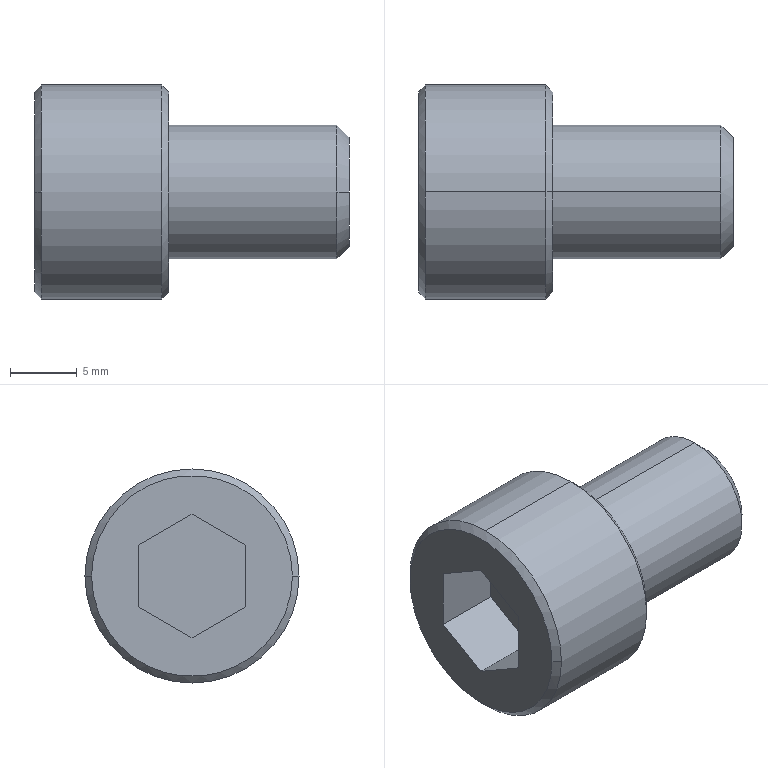Part | STEP file | TR_32x10-5 | 1 solid | 20 faces | box 23.5 x 16 x 16 mm | volume 2769 mm3 | plane 10 | cone 6 | cylinder 4 | commonest cylinder face diameters 10 x2 16 x2
STEP:
#1=CARTESIAN_POINT('',(0.,0.,0.));
#2=DIRECTION('',(0.,0.,1.));
#3=DIRECTION('',(1.,0.,0.));
#4=AXIS2_PLACEMENT_3D('',#1,#2,#3);
#5=CARTESIAN_POINT('',(-29.5,-14.,19.));
#6=VERTEX_POINT('',#5);
#7=CARTESIAN_POINT('',(-29.5,-22.,27.));
#8=VERTEX_POINT('',#7);
#9=CARTESIAN_POINT('',(-29.5,-22.,19.));
#10=DIRECTION('',(1.,0.,0.));
#11=DIRECTION('',(0.,0.,-1.));
#12=AXIS2_PLACEMENT_3D('',#9,#10,#11);
#13=CIRCLE('',#12,8.);
#14=CARTESIAN_POINT('',(-25.,-22.,19.));
#15=DIRECTION('',(1.,0.,0.));
#16=DIRECTION('',(0.,0.,-1.));
#17=AXIS2_PLACEMENT_3D('',#14,#15,#16);
#18=CYLINDRICAL_SURFACE('',#17,8.);
#19=CARTESIAN_POINT('',(0.,-4.5));
#20=DIRECTION('',(1.,0.));
#21=VECTOR('',#20,1.);
#22=LINE('',#19,#21);
#23=(GEOMETRIC_REPRESENTATION_CONTEXT(2)PARAMETRIC_REPRESENTATION_CONTEXT()REPRESENTATION_CONTEXT('',''));
#24=DEFINITIONAL_REPRESENTATION('',(#22),#23);
#25=PCURVE('',#18,#24);
#26=CARTESIAN_POINT('',(-29.5,-22.,19.));
#27=DIRECTION('',(1.,0.,0.));
#28=DIRECTION('',(0.,1.,0.));
#29=AXIS2_PLACEMENT_3D('',#26,#27,#28);
#30=CONICAL_SURFACE('',#29,8.,0.7854);
#31=CARTESIAN_POINT('',(-1.571,0.));
#32=DIRECTION('',(1.,0.));
#33=VECTOR('',#32,1.);
#34=LINE('',#31,#33);
#35=(GEOMETRIC_REPRESENTATION_CONTEXT(2)PARAMETRIC_REPRESENTATION_CONTEXT()REPRESENTATION_CONTEXT('',''));
#36=DEFINITIONAL_REPRESENTATION('',(#34),#35);
#37=PCURVE('',#30,#36);
#38=SURFACE_CURVE('',#13,(#25,#37),.PCURVE_S1.);
#39=EDGE_CURVE('',#6,#8,#38,.T.);
#40=ORIENTED_EDGE('',*,*,#39,.T.);
#41=CARTESIAN_POINT('',(-20.5,-22.,27.));
#42=VERTEX_POINT('',#41);
#43=CARTESIAN_POINT('',(-25.,-22.,27.));
#44=DIRECTION('',(1.,0.,0.));
#45=VECTOR('',#44,1.);
#46=LINE('',#43,#45);
#47=CARTESIAN_POINT('',(3.142,0.));
#48=DIRECTION('',(0.,1.));
#49=VECTOR('',#48,1.);
#50=LINE('',#47,#49);
#51=(GEOMETRIC_REPRESENTATION_CONTEXT(2)PARAMETRIC_REPRESENTATION_CONTEXT()REPRESENTATION_CONTEXT('',''));
#52=DEFINITIONAL_REPRESENTATION('',(#50),#51);
#53=PCURVE('',#18,#52);
#54=CARTESIAN_POINT('',(-25.,-22.,19.));
#55=DIRECTION('',(1.,0.,0.));
#56=DIRECTION('',(0.,0.,-1.));
#57=AXIS2_PLACEMENT_3D('',#54,#55,#56);
#58=CYLINDRICAL_SURFACE('',#57,8.);
#59=CARTESIAN_POINT('',(3.142,0.));
#60=DIRECTION('',(0.,1.));
#61=VECTOR('',#60,1.);
#62=LINE('',#59,#61);
#63=(GEOMETRIC_REPRESENTATION_CONTEXT(2)PARAMETRIC_REPRESENTATION_CONTEXT()REPRESENTATION_CONTEXT('',''));
#64=DEFINITIONAL_REPRESENTATION('',(#62),#63);
#65=PCURVE('',#58,#64);
#66=SURFACE_CURVE('',#46,(#53,#65),.PCURVE_S1.);
#67=EDGE_CURVE('',#8,#42,#66,.T.);
#68=ORIENTED_EDGE('',*,*,#67,.T.);
#69=CARTESIAN_POINT('',(-20.5,-22.,11.));
#70=VERTEX_POINT('',#69);
#71=CARTESIAN_POINT('',(-20.5,-22.,19.));
#72=DIRECTION('',(-1.,0.,0.));
#73=DIRECTION('',(0.,0.,-1.));
#74=AXIS2_PLACEMENT_3D('',#71,#72,#73);
#75=CIRCLE('',#74,8.);
#76=CARTESIAN_POINT('',(6.283,4.5));
#77=DIRECTION('',(-1.,0.));
#78=VECTOR('',#77,1.);
#79=LINE('',#76,#78);
#80=(GEOMETRIC_REPRESENTATION_CONTEXT(2)PARAMETRIC_REPRESENTATION_CONTEXT()REPRESENTATION_CONTEXT('',''));
#81=DEFINITIONAL_REPRESENTATION('',(#79),#80);
#82=PCURVE('',#18,#81);
#83=CARTESIAN_POINT('',(-20.5,-22.,19.));
#84=DIRECTION('',(-1.,0.,0.));
#85=DIRECTION('',(0.,0.,1.));
#86=AXIS2_PLACEMENT_3D('',#83,#84,#85);
#87=CONICAL_SURFACE('',#86,8.,0.7854);
#88=CARTESIAN_POINT('',(-3.142,0.));
#89=DIRECTION('',(1.,0.));
#90=VECTOR('',#89,1.);
#91=LINE('',#88,#90);
#92=(GEOMETRIC_REPRESENTATION_CONTEXT(2)PARAMETRIC_REPRESENTATION_CONTEXT()REPRESENTATION_CONTEXT('',''));
#93=DEFINITIONAL_REPRESENTATION('',(#91),#92);
#94=PCURVE('',#87,#93);
#95=SURFACE_CURVE('',#75,(#82,#94),.PCURVE_S1.);
#96=EDGE_CURVE('',#42,#70,#95,.T.);
#97=ORIENTED_EDGE('',*,*,#96,.T.);
#98=CARTESIAN_POINT('',(-29.5,-22.,11.));
#99=VERTEX_POINT('',#98);
#100=CARTESIAN_POINT('',(-25.,-22.,11.));
#101=DIRECTION('',(1.,0.,0.));
#102=VECTOR('',#101,1.);
#103=LINE('',#100,#102);
#104=CARTESIAN_POINT('',(0.,0.));
#105=DIRECTION('',(0.,1.));
#106=VECTOR('',#105,1.);
#107=LINE('',#104,#106);
#108=(GEOMETRIC_REPRESENTATION_CONTEXT(2)PARAMETRIC_REPRESENTATION_CONTEXT()REPRESENTATION_CONTEXT('',''));
#109=DEFINITIONAL_REPRESENTATION('',(#107),#108);
#110=PCURVE('',#18,#109);
#111=CARTESIAN_POINT('',(6.283,0.));
#112=DIRECTION('',(0.,1.));
#113=VECTOR('',#112,1.);
#114=LINE('',#111,#113);
#115=(GEOMETRIC_REPRESENTATION_CONTEXT(2)PARAMETRIC_REPRESENTATION_CONTEXT()REPRESENTATION_CONTEXT('',''));
#116=DEFINITIONAL_REPRESENTATION('',(#114),#115);
#117=PCURVE('',#58,#116);
#118=SURFACE_CURVE('',#103,(#110,#117),.PCURVE_S1.);
#119=EDGE_CURVE('',#99,#70,#118,.T.);
#120=ORIENTED_EDGE('',*,*,#119,.F.);
#121=CARTESIAN_POINT('',(-29.5,-22.,19.));
#122=DIRECTION('',(1.,0.,0.));
#123=DIRECTION('',(0.,0.,-1.));
#124=AXIS2_PLACEMENT_3D('',#121,#122,#123);
#125=CIRCLE('',#124,8.);
#126=CARTESIAN_POINT('',(0.,-4.5));
#127=DIRECTION('',(1.,0.));
#128=VECTOR('',#127,1.);
#129=LINE('',#126,#128);
#130=(GEOMETRIC_REPRESENTATION_CONTEXT(2)PARAMETRIC_REPRESENTATION_CONTEXT()REPRESENTATION_CONTEXT('',''));
#131=DEFINITIONAL_REPRESENTATION('',(#129),#130);
#132=PCURVE('',#18,#131);
#133=CARTESIAN_POINT('',(-29.5,-22.,19.));
#134=DIRECTION('',(1.,0.,0.));
#135=DIRECTION('',(0.,1.,0.));
#136=AXIS2_PLACEMENT_3D('',#133,#134,#135);
#137=CONICAL_SURFACE('',#136,8.,0.7854);
#138=CARTESIAN_POINT('',(4.712,0.));
#139=DIRECTION('',(1.,0.));
#140=VECTOR('',#139,1.);
#141=LINE('',#138,#140);
#142=(GEOMETRIC_REPRESENTATION_CONTEXT(2)PARAMETRIC_REPRESENTATION_CONTEXT()REPRESENTATION_CONTEXT('',''));
#143=DEFINITIONAL_REPRESENTATION('',(#141),#142);
#144=PCURVE('',#137,#143);
#145=SURFACE_CURVE('',#125,(#132,#144),.PCURVE_S1.);
#146=EDGE_CURVE('',#99,#6,#145,.T.);
#147=ORIENTED_EDGE('',*,*,#146,.T.);
#148=EDGE_LOOP('',(#40,#68,#97,#120,#147));
#149=FACE_BOUND('',#148,.T.);
#150=ADVANCED_FACE('',(#149),#18,.T.);
#151=CARTESIAN_POINT('',(-30.,-14.5,19.));
#152=VERTEX_POINT('',#151);
#153=CARTESIAN_POINT('',(-30.,-29.5,19.));
#154=VERTEX_POINT('',#153);
#155=CARTESIAN_POINT('',(-30.,-22.,19.));
#156=DIRECTION('',(1.,0.,0.));
#157=DIRECTION('',(0.,1.,0.));
#158=AXIS2_PLACEMENT_3D('',#155,#156,#157);
#159=CIRCLE('',#158,7.5);
#160=CARTESIAN_POINT('',(0.,-0.5));
#161=DIRECTION('',(1.,0.));
#162=VECTOR('',#161,1.);
#163=LINE('',#160,#162);
#164=(GEOMETRIC_REPRESENTATION_CONTEXT(2)PARAMETRIC_REPRESENTATION_CONTEXT()REPRESENTATION_CONTEXT('',''));
#165=DEFINITIONAL_REPRESENTATION('',(#163),#164);
#166=PCURVE('',#30,#165);
#167=CARTESIAN_POINT('',(-30.,-22.,22.75));
#168=DIRECTION('',(-1.,0.,0.));
#169=DIRECTION('',(0.,0.,1.));
#170=AXIS2_PLACEMENT_3D('',#167,#168,#169);
#171=PLANE('',#170);
#172=CARTESIAN_POINT('',(-3.75,7.5));
#173=CARTESIAN_POINT('',(9.24,7.5));
#174=CARTESIAN_POINT('',(2.745,-3.75));
#175=CARTESIAN_POINT('',(-3.75,-15.));
#176=CARTESIAN_POINT('',(-10.245,-3.75));
#177=CARTESIAN_POINT('',(-16.74,7.5));
#178=CARTESIAN_POINT('',(-3.75,7.5));
#179=(BOUNDED_CURVE()B_SPLINE_CURVE(2,(#172,#173,#174,#175,#176,#177,#178),.UNSPECIFIED.,.T.,.F.)B_SPLINE_CURVE_WITH_KNOTS((1,2,2,2,2,1),(-2.094,0.,2.094,4.189,6.283,8.378),.UNSPECIFIED.)CURVE()GEOMETRIC_REPRESENTATION_ITEM()RATIONAL_B_SPLINE_CURVE((1.,0.5,1.,0.5,1.,0.5,1.))REPRESENTATION_ITEM(''));
#180=(GEOMETRIC_REPRESENTATION_CONTEXT(2)PARAMETRIC_REPRESENTATION_CONTEXT()REPRESENTATION_CONTEXT('',''));
#181=DEFINITIONAL_REPRESENTATION('',(#179),#180);
#182=PCURVE('',#171,#181);
#183=SURFACE_CURVE('',#159,(#166,#182),.PCURVE_S1.);
#184=EDGE_CURVE('',#152,#154,#183,.T.);
#185=ORIENTED_EDGE('',*,*,#184,.T.);
#186=CARTESIAN_POINT('',(-29.5,-30.,19.));
#187=VERTEX_POINT('',#186);
#188=CARTESIAN_POINT('',(-29.5,-30.,19.));
#189=DIRECTION('',(0.7071,-0.7071,0.));
#190=VECTOR('',#189,1.);
#191=LINE('',#188,#190);
#192=CARTESIAN_POINT('',(3.142,0.));
#193=DIRECTION('',(0.,1.));
#194=VECTOR('',#193,1.);
#195=LINE('',#192,#194);
#196=(GEOMETRIC_REPRESENTATION_CONTEXT(2)PARAMETRIC_REPRESENTATION_CONTEXT()REPRESENTATION_CONTEXT('',''));
#197=DEFINITIONAL_REPRESENTATION('',(#195),#196);
#198=PCURVE('',#30,#197);
#199=CARTESIAN_POINT('',(3.142,0.));
#200=DIRECTION('',(0.,1.));
#201=VECTOR('',#200,1.);
#202=LINE('',#199,#201);
#203=(GEOMETRIC_REPRESENTATION_CONTEXT(2)PARAMETRIC_REPRESENTATION_CONTEXT()REPRESENTATION_CONTEXT('',''));
#204=DEFINITIONAL_REPRESENTATION('',(#202),#203);
#205=PCURVE('',#137,#204);
#206=SURFACE_CURVE('',#191,(#198,#205),.PCURVE_S1.);
#207=EDGE_CURVE('',#154,#187,#206,.T.);
#208=ORIENTED_EDGE('',*,*,#207,.T.);
#209=CARTESIAN_POINT('',(-29.5,-22.,19.));
#210=DIRECTION('',(1.,0.,0.));
#211=DIRECTION('',(0.,0.,-1.));
#212=AXIS2_PLACEMENT_3D('',#209,#210,#211);
#213=CIRCLE('',#212,8.);
#214=CARTESIAN_POINT('',(-1.571,0.));
#215=DIRECTION('',(1.,0.));
#216=VECTOR('',#215,1.);
#217=LINE('',#214,#216);
#218=(GEOMETRIC_REPRESENTATION_CONTEXT(2)PARAMETRIC_REPRESENTATION_CONTEXT()REPRESENTATION_CONTEXT('',''));
#219=DEFINITIONAL_REPRESENTATION('',(#217),#218);
#220=PCURVE('',#30,#219);
#221=CARTESIAN_POINT('',(0.,-4.5));
#222=DIRECTION('',(1.,0.));
#223=VECTOR('',#222,1.);
#224=LINE('',#221,#223);
#225=(GEOMETRIC_REPRESENTATION_CONTEXT(2)PARAMETRIC_REPRESENTATION_CONTEXT()REPRESENTATION_CONTEXT('',''));
#226=DEFINITIONAL_REPRESENTATION('',(#224),#225);
#227=PCURVE('',#58,#226);
#228=SURFACE_CURVE('',#213,(#220,#227),.PCURVE_S1.);
#229=EDGE_CURVE('',#8,#187,#228,.T.);
#230=ORIENTED_EDGE('',*,*,#229,.F.);
#231=ORIENTED_EDGE('',*,*,#39,.F.);
#232=CARTESIAN_POINT('',(-29.5,-14.,19.));
#233=DIRECTION('',(0.7071,0.7071,0.));
#234=VECTOR('',#233,1.);
#235=LINE('',#232,#234);
#236=CARTESIAN_POINT('',(0.,0.));
#237=DIRECTION('',(0.,1.));
#238=VECTOR('',#237,1.);
#239=LINE('',#236,#238);
#240=(GEOMETRIC_REPRESENTATION_CONTEXT(2)PARAMETRIC_REPRESENTATION_CONTEXT()REPRESENTATION_CONTEXT('',''));
#241=DEFINITIONAL_REPRESENTATION('',(#239),#240);
#242=PCURVE('',#30,#241);
#243=CARTESIAN_POINT('',(6.283,0.));
#244=DIRECTION('',(0.,1.));
#245=VECTOR('',#244,1.);
#246=LINE('',#243,#245);
#247=(GEOMETRIC_REPRESENTATION_CONTEXT(2)PARAMETRIC_REPRESENTATION_CONTEXT()REPRESENTATION_CONTEXT('',''));
#248=DEFINITIONAL_REPRESENTATION('',(#246),#247);
#249=PCURVE('',#137,#248);
#250=SURFACE_CURVE('',#235,(#242,#249),.PCURVE_S1.);
#251=EDGE_CURVE('',#152,#6,#250,.T.);
#252=ORIENTED_EDGE('',*,*,#251,.F.);
#253=EDGE_LOOP('',(#185,#208,#230,#231,#252));
#254=FACE_BOUND('',#253,.T.);
#255=ADVANCED_FACE('',(#254),#30,.T.);
#256=CARTESIAN_POINT('',(-20.,-22.,26.5));
#257=VERTEX_POINT('',#256);
#258=CARTESIAN_POINT('',(-20.,-22.,11.5));
#259=VERTEX_POINT('',#258);
#260=CARTESIAN_POINT('',(-20.,-22.,19.));
#261=DIRECTION('',(-1.,0.,0.));
#262=DIRECTION('',(0.,0.,1.));
#263=AXIS2_PLACEMENT_3D('',#260,#261,#262);
#264=CIRCLE('',#263,7.5);
#265=CARTESIAN_POINT('',(0.,-0.5));
#266=DIRECTION('',(1.,0.));
#267=VECTOR('',#266,1.);
#268=LINE('',#265,#267);
#269=(GEOMETRIC_REPRESENTATION_CONTEXT(2)PARAMETRIC_REPRESENTATION_CONTEXT()REPRESENTATION_CONTEXT('',''));
#270=DEFINITIONAL_REPRESENTATION('',(#268),#269);
#271=PCURVE('',#87,#270);
#272=CARTESIAN_POINT('',(-20.,-22.,25.25));
#273=DIRECTION('',(1.,0.,0.));
#274=DIRECTION('',(0.,0.,-1.));
#275=AXIS2_PLACEMENT_3D('',#272,#273,#274);
#276=PLANE('',#275);
#277=CARTESIAN_POINT('',(-1.25,0.));
#278=CARTESIAN_POINT('',(-1.25,12.99));
#279=CARTESIAN_POINT('',(10.,6.495));
#280=CARTESIAN_POINT('',(21.25,0.));
#281=CARTESIAN_POINT('',(10.,-6.495));
#282=CARTESIAN_POINT('',(-1.25,-12.99));
#283=CARTESIAN_POINT('',(-1.25,0.));
#284=(BOUNDED_CURVE()B_SPLINE_CURVE(2,(#277,#278,#279,#280,#281,#282,#283),.UNSPECIFIED.,.T.,.F.)B_SPLINE_CURVE_WITH_KNOTS((1,2,2,2,2,1),(-2.094,0.,2.094,4.189,6.283,8.378),.UNSPECIFIED.)CURVE()GEOMETRIC_REPRESENTATION_ITEM()RATIONAL_B_SPLINE_CURVE((1.,0.5,1.,0.5,1.,0.5,1.))REPRESENTATION_ITEM(''));
#285=(GEOMETRIC_REPRESENTATION_CONTEXT(2)PARAMETRIC_REPRESENTATION_CONTEXT()REPRESENTATION_CONTEXT('',''));
#286=DEFINITIONAL_REPRESENTATION('',(#284),#285);
#287=PCURVE('',#276,#286);
#288=SURFACE_CURVE('',#264,(#271,#287),.PCURVE_S1.);
#289=EDGE_CURVE('',#257,#259,#288,.T.);
#290=ORIENTED_EDGE('',*,*,#289,.T.);
#291=CARTESIAN_POINT('',(-20.5,-22.,11.));
#292=DIRECTION('',(-0.7071,0.,-0.7071));
#293=VECTOR('',#292,1.);
#294=LINE('',#291,#293);
#295=CARTESIAN_POINT('',(3.142,0.));
#296=DIRECTION('',(0.,1.));
#297=VECTOR('',#296,1.);
#298=LINE('',#295,#297);
#299=(GEOMETRIC_REPRESENTATION_CONTEXT(2)PARAMETRIC_REPRESENTATION_CONTEXT()REPRESENTATION_CONTEXT('',''));
#300=DEFINITIONAL_REPRESENTATION('',(#298),#299);
#301=PCURVE('',#87,#300);
#302=CARTESIAN_POINT('',(-20.5,-22.,19.));
#303=DIRECTION('',(-1.,0.,0.));
#304=DIRECTION('',(0.,0.,1.));
#305=AXIS2_PLACEMENT_3D('',#302,#303,#304);
#306=CONICAL_SURFACE('',#305,8.,0.7854);
#307=CARTESIAN_POINT('',(3.142,0.));
#308=DIRECTION('',(0.,1.));
#309=VECTOR('',#308,1.);
#310=LINE('',#307,#309);
#311=(GEOMETRIC_REPRESENTATION_CONTEXT(2)PARAMETRIC_REPRESENTATION_CONTEXT()REPRESENTATION_CONTEXT('',''));
#312=DEFINITIONAL_REPRESENTATION('',(#310),#311);
#313=PCURVE('',#306,#312);
#314=SURFACE_CURVE('',#294,(#301,#313),.PCURVE_S1.);
#315=EDGE_CURVE('',#259,#70,#314,.T.);
#316=ORIENTED_EDGE('',*,*,#315,.T.);
#317=ORIENTED_EDGE('',*,*,#96,.F.);
#318=CARTESIAN_POINT('',(-20.5,-22.,27.));
#319=DIRECTION('',(-0.7071,0.,0.7071));
#320=VECTOR('',#319,1.);
#321=LINE('',#318,#320);
#322=CARTESIAN_POINT('',(0.,0.));
#323=DIRECTION('',(0.,1.));
#324=VECTOR('',#323,1.);
#325=LINE('',#322,#324);
#326=(GEOMETRIC_REPRESENTATION_CONTEXT(2)PARAMETRIC_REPRESENTATION_CONTEXT()REPRESENTATION_CONTEXT('',''));
#327=DEFINITIONAL_REPRESENTATION('',(#325),#326);
#328=PCURVE('',#87,#327);
#329=CARTESIAN_POINT('',(6.283,0.));
#330=DIRECTION('',(0.,1.));
#331=VECTOR('',#330,1.);
#332=LINE('',#329,#331);
#333=(GEOMETRIC_REPRESENTATION_CONTEXT(2)PARAMETRIC_REPRESENTATION_CONTEXT()REPRESENTATION_CONTEXT('',''));
#334=DEFINITIONAL_REPRESENTATION('',(#332),#333);
#335=PCURVE('',#306,#334);
#336=SURFACE_CURVE('',#321,(#328,#335),.PCURVE_S1.);
#337=EDGE_CURVE('',#257,#42,#336,.T.);
#338=ORIENTED_EDGE('',*,*,#337,.F.);
#339=EDGE_LOOP('',(#290,#316,#317,#338));
#340=FACE_BOUND('',#339,.T.);
#341=ADVANCED_FACE('',(#340),#87,.T.);
#342=CARTESIAN_POINT('',(-20.,-22.,24.));
#343=VERTEX_POINT('',#342);
#344=CARTESIAN_POINT('',(-20.,-22.,14.));
#345=VERTEX_POINT('',#344);
#346=CARTESIAN_POINT('',(-20.,-22.,19.));
#347=DIRECTION('',(-1.,0.,0.));
#348=DIRECTION('',(0.,0.,-1.));
#349=AXIS2_PLACEMENT_3D('',#346,#347,#348);
#350=CIRCLE('',#349,5.);
#351=CARTESIAN_POINT('',(-13.71,-22.,19.));
#352=DIRECTION('',(1.,0.,0.));
#353=DIRECTION('',(0.,0.,-1.));
#354=AXIS2_PLACEMENT_3D('',#351,#352,#353);
#355=CYLINDRICAL_SURFACE('',#354,5.);
#356=CARTESIAN_POINT('',(6.283,-6.29));
#357=DIRECTION('',(-1.,0.));
#358=VECTOR('',#357,1.);
#359=LINE('',#356,#358);
#360=(GEOMETRIC_REPRESENTATION_CONTEXT(2)PARAMETRIC_REPRESENTATION_CONTEXT()REPRESENTATION_CONTEXT('',''));
#361=DEFINITIONAL_REPRESENTATION('',(#359),#360);
#362=PCURVE('',#355,#361);
#363=CARTESIAN_POINT('',(11.25,0.));
#364=CARTESIAN_POINT('',(11.25,-8.66));
#365=CARTESIAN_POINT('',(3.75,-4.33));
#366=CARTESIAN_POINT('',(-3.75,0.));
#367=CARTESIAN_POINT('',(3.75,4.33));
#368=CARTESIAN_POINT('',(11.25,8.66));
#369=CARTESIAN_POINT('',(11.25,0.));
#370=(BOUNDED_CURVE()B_SPLINE_CURVE(2,(#363,#364,#365,#366,#367,#368,#369),.UNSPECIFIED.,.T.,.F.)B_SPLINE_CURVE_WITH_KNOTS((1,2,2,2,2,1),(-2.094,0.,2.094,4.189,6.283,8.378),.UNSPECIFIED.)CURVE()GEOMETRIC_REPRESENTATION_ITEM()RATIONAL_B_SPLINE_CURVE((1.,0.5,1.,0.5,1.,0.5,1.))REPRESENTATION_ITEM(''));
#371=(GEOMETRIC_REPRESENTATION_CONTEXT(2)PARAMETRIC_REPRESENTATION_CONTEXT()REPRESENTATION_CONTEXT('',''));
#372=DEFINITIONAL_REPRESENTATION('',(#370),#371);
#373=PCURVE('',#276,#372);
#374=SURFACE_CURVE('',#350,(#362,#373),.PCURVE_S1.);
#375=EDGE_CURVE('',#343,#345,#374,.T.);
#376=ORIENTED_EDGE('',*,*,#375,.F.);
#377=CARTESIAN_POINT('',(-7.42,-22.,24.));
#378=VERTEX_POINT('',#377);
#379=CARTESIAN_POINT('',(-13.71,-22.,24.));
#380=DIRECTION('',(1.,0.,0.));
#381=VECTOR('',#380,1.);
#382=LINE('',#379,#381);
#383=CARTESIAN_POINT('',(3.142,0.));
#384=DIRECTION('',(0.,1.));
#385=VECTOR('',#384,1.);
#386=LINE('',#383,#385);
#387=(GEOMETRIC_REPRESENTATION_CONTEXT(2)PARAMETRIC_REPRESENTATION_CONTEXT()REPRESENTATION_CONTEXT('',''));
#388=DEFINITIONAL_REPRESENTATION('',(#386),#387);
#389=PCURVE('',#355,#388);
#390=CARTESIAN_POINT('',(-13.71,-22.,19.));
#391=DIRECTION('',(1.,0.,0.));
#392=DIRECTION('',(0.,0.,-1.));
#393=AXIS2_PLACEMENT_3D('',#390,#391,#392);
#394=CYLINDRICAL_SURFACE('',#393,5.);
#395=CARTESIAN_POINT('',(3.142,0.));
#396=DIRECTION('',(0.,1.));
#397=VECTOR('',#396,1.);
#398=LINE('',#395,#397);
#399=(GEOMETRIC_REPRESENTATION_CONTEXT(2)PARAMETRIC_REPRESENTATION_CONTEXT()REPRESENTATION_CONTEXT('',''));
#400=DEFINITIONAL_REPRESENTATION('',(#398),#399);
#401=PCURVE('',#394,#400);
#402=SURFACE_CURVE('',#382,(#389,#401),.PCURVE_S1.);
#403=EDGE_CURVE('',#343,#378,#402,.T.);
#404=ORIENTED_EDGE('',*,*,#403,.T.);
#405=CARTESIAN_POINT('',(-7.42,-17.,19.));
#406=VERTEX_POINT('',#405);
#407=CARTESIAN_POINT('',(-7.42,-22.,19.));
#408=DIRECTION('',(-1.,0.,0.));
#409=DIRECTION('',(0.,0.,-1.));
#410=AXIS2_PLACEMENT_3D('',#407,#408,#409);
#411=CIRCLE('',#410,5.);
#412=CARTESIAN_POINT('',(6.283,6.29));
#413=DIRECTION('',(-1.,0.));
#414=VECTOR('',#413,1.);
#415=LINE('',#412,#414);
#416=(GEOMETRIC_REPRESENTATION_CONTEXT(2)PARAMETRIC_REPRESENTATION_CONTEXT()REPRESENTATION_CONTEXT('',''));
#417=DEFINITIONAL_REPRESENTATION('',(#415),#416);
#418=PCURVE('',#355,#417);
#419=CARTESIAN_POINT('',(-7.42,-22.,19.));
#420=DIRECTION('',(-1.,0.,0.));
#421=DIRECTION('',(0.,-1.,0.));
#422=AXIS2_PLACEMENT_3D('',#419,#420,#421);
#423=CONICAL_SURFACE('',#422,5.,0.7854);
#424=CARTESIAN_POINT('',(-1.571,0.));
#425=DIRECTION('',(1.,0.));
#426=VECTOR('',#425,1.);
#427=LINE('',#424,#426);
#428=(GEOMETRIC_REPRESENTATION_CONTEXT(2)PARAMETRIC_REPRESENTATION_CONTEXT()REPRESENTATION_CONTEXT('',''));
#429=DEFINITIONAL_REPRESENTATION('',(#427),#428);
#430=PCURVE('',#423,#429);
#431=SURFACE_CURVE('',#411,(#418,#430),.PCURVE_S1.);
#432=EDGE_CURVE('',#378,#406,#431,.T.);
#433=ORIENTED_EDGE('',*,*,#432,.T.);
#434=CARTESIAN_POINT('',(-7.42,-22.,14.));
#435=VERTEX_POINT('',#434);
#436=CARTESIAN_POINT('',(-7.42,-22.,19.));
#437=DIRECTION('',(-1.,0.,0.));
#438=DIRECTION('',(0.,0.,-1.));
#439=AXIS2_PLACEMENT_3D('',#436,#437,#438);
#440=CIRCLE('',#439,5.);
#441=CARTESIAN_POINT('',(6.283,6.29));
#442=DIRECTION('',(-1.,0.));
#443=VECTOR('',#442,1.);
#444=LINE('',#441,#443);
#445=(GEOMETRIC_REPRESENTATION_CONTEXT(2)PARAMETRIC_REPRESENTATION_CONTEXT()REPRESENTATION_CONTEXT('',''));
#446=DEFINITIONAL_REPRESENTATION('',(#444),#445);
#447=PCURVE('',#355,#446);
#448=CARTESIAN_POINT('',(-7.42,-22.,19.));
#449=DIRECTION('',(-1.,0.,0.));
#450=DIRECTION('',(0.,-1.,0.));
#451=AXIS2_PLACEMENT_3D('',#448,#449,#450);
#452=CONICAL_SURFACE('',#451,5.,0.7854);
#453=CARTESIAN_POINT('',(-1.571,0.));
#454=DIRECTION('',(1.,0.));
#455=VECTOR('',#454,1.);
#456=LINE('',#453,#455);
#457=(GEOMETRIC_REPRESENTATION_CONTEXT(2)PARAMETRIC_REPRESENTATION_CONTEXT()REPRESENTATION_CONTEXT('',''));
#458=DEFINITIONAL_REPRESENTATION('',(#456),#457);
#459=PCURVE('',#452,#458);
#460=SURFACE_CURVE('',#440,(#447,#459),.PCURVE_S1.);
#461=EDGE_CURVE('',#406,#435,#460,.T.);
#462=ORIENTED_EDGE('',*,*,#461,.T.);
#463=CARTESIAN_POINT('',(-13.71,-22.,14.));
#464=DIRECTION('',(1.,0.,0.));
#465=VECTOR('',#464,1.);
#466=LINE('',#463,#465);
#467=CARTESIAN_POINT('',(0.,0.));
#468=DIRECTION('',(0.,1.));
#469=VECTOR('',#468,1.);
#470=LINE('',#467,#469);
#471=(GEOMETRIC_REPRESENTATION_CONTEXT(2)PARAMETRIC_REPRESENTATION_CONTEXT()REPRESENTATION_CONTEXT('',''));
#472=DEFINITIONAL_REPRESENTATION('',(#470),#471);
#473=PCURVE('',#355,#472);
#474=CARTESIAN_POINT('',(6.283,0.));
#475=DIRECTION('',(0.,1.));
#476=VECTOR('',#475,1.);
#477=LINE('',#474,#476);
#478=(GEOMETRIC_REPRESENTATION_CONTEXT(2)PARAMETRIC_REPRESENTATION_CONTEXT()REPRESENTATION_CONTEXT('',''));
#479=DEFINITIONAL_REPRESENTATION('',(#477),#478);
#480=PCURVE('',#394,#479);
#481=SURFACE_CURVE('',#466,(#473,#480),.PCURVE_S1.);
#482=EDGE_CURVE('',#345,#435,#481,.T.);
#483=ORIENTED_EDGE('',*,*,#482,.F.);
#484=EDGE_LOOP('',(#376,#404,#433,#462,#483));
#485=FACE_BOUND('',#484,.T.);
#486=ADVANCED_FACE('',(#485),#355,.T.);
#487=CARTESIAN_POINT('',(-6.5,-26.08,19.));
#488=VERTEX_POINT('',#487);
#489=CARTESIAN_POINT('',(-6.5,-17.92,19.));
#490=VERTEX_POINT('',#489);
#491=CARTESIAN_POINT('',(-6.5,-22.,19.));
#492=DIRECTION('',(-1.,0.,0.));
#493=DIRECTION('',(0.,-1.,0.));
#494=AXIS2_PLACEMENT_3D('',#491,#492,#493);
#495=CIRCLE('',#494,4.08);
#496=CARTESIAN_POINT('',(0.,-0.92));
#497=DIRECTION('',(1.,0.));
#498=VECTOR('',#497,1.);
#499=LINE('',#496,#498);
#500=(GEOMETRIC_REPRESENTATION_CONTEXT(2)PARAMETRIC_REPRESENTATION_CONTEXT()REPRESENTATION_CONTEXT('',''));
#501=DEFINITIONAL_REPRESENTATION('',(#499),#500);
#502=PCURVE('',#423,#501);
#503=CARTESIAN_POINT('',(-6.5,-22.,21.04));
#504=DIRECTION('',(1.,0.,0.));
#505=DIRECTION('',(0.,0.,-1.));
#506=AXIS2_PLACEMENT_3D('',#503,#504,#505);
#507=PLANE('',#506);
#508=CARTESIAN_POINT('',(2.04,-4.08));
#509=CARTESIAN_POINT('',(-5.027,-4.08));
#510=CARTESIAN_POINT('',(-1.493,2.04));
#511=CARTESIAN_POINT('',(2.04,8.16));
#512=CARTESIAN_POINT('',(5.573,2.04));
#513=CARTESIAN_POINT('',(9.107,-4.08));
#514=CARTESIAN_POINT('',(2.04,-4.08));
#515=(BOUNDED_CURVE()B_SPLINE_CURVE(2,(#508,#509,#510,#511,#512,#513,#514),.UNSPECIFIED.,.T.,.F.)B_SPLINE_CURVE_WITH_KNOTS((1,2,2,2,2,1),(-2.094,0.,2.094,4.189,6.283,8.378),.UNSPECIFIED.)CURVE()GEOMETRIC_REPRESENTATION_ITEM()RATIONAL_B_SPLINE_CURVE((1.,0.5,1.,0.5,1.,0.5,1.))REPRESENTATION_ITEM(''));
#516=(GEOMETRIC_REPRESENTATION_CONTEXT(2)PARAMETRIC_REPRESENTATION_CONTEXT()REPRESENTATION_CONTEXT('',''));
#517=DEFINITIONAL_REPRESENTATION('',(#515),#516);
#518=PCURVE('',#507,#517);
#519=SURFACE_CURVE('',#495,(#502,#518),.PCURVE_S1.);
#520=EDGE_CURVE('',#488,#490,#519,.T.);
#521=ORIENTED_EDGE('',*,*,#520,.T.);
#522=CARTESIAN_POINT('',(-7.42,-17.,19.));
#523=DIRECTION('',(-0.7071,0.7071,0.));
#524=VECTOR('',#523,1.);
#525=LINE('',#522,#524);
#526=CARTESIAN_POINT('',(3.142,0.));
#527=DIRECTION('',(0.,1.));
#528=VECTOR('',#527,1.);
#529=LINE('',#526,#528);
#530=(GEOMETRIC_REPRESENTATION_CONTEXT(2)PARAMETRIC_REPRESENTATION_CONTEXT()REPRESENTATION_CONTEXT('',''));
#531=DEFINITIONAL_REPRESENTATION('',(#529),#530);
#532=PCURVE('',#423,#531);
#533=CARTESIAN_POINT('',(3.142,0.));
#534=DIRECTION('',(0.,1.));
#535=VECTOR('',#534,1.);
#536=LINE('',#533,#535);
#537=(GEOMETRIC_REPRESENTATION_CONTEXT(2)PARAMETRIC_REPRESENTATION_CONTEXT()REPRESENTATION_CONTEXT('',''));
#538=DEFINITIONAL_REPRESENTATION('',(#536),#537);
#539=PCURVE('',#452,#538);
#540=SURFACE_CURVE('',#525,(#532,#539),.PCURVE_S1.);
#541=EDGE_CURVE('',#490,#406,#540,.T.);
#542=ORIENTED_EDGE('',*,*,#541,.T.);
#543=ORIENTED_EDGE('',*,*,#432,.F.);
#544=CARTESIAN_POINT('',(-7.42,-27.,19.));
#545=VERTEX_POINT('',#544);
#546=CARTESIAN_POINT('',(-7.42,-22.,19.));
#547=DIRECTION('',(-1.,0.,0.));
#548=DIRECTION('',(0.,0.,-1.));
#549=AXIS2_PLACEMENT_3D('',#546,#547,#548);
#550=CIRCLE('',#549,5.);
#551=CARTESIAN_POINT('',(-1.571,0.));
#552=DIRECTION('',(1.,0.));
#553=VECTOR('',#552,1.);
#554=LINE('',#551,#553);
#555=(GEOMETRIC_REPRESENTATION_CONTEXT(2)PARAMETRIC_REPRESENTATION_CONTEXT()REPRESENTATION_CONTEXT('',''));
#556=DEFINITIONAL_REPRESENTATION('',(#554),#555);
#557=PCURVE('',#423,#556);
#558=CARTESIAN_POINT('',(6.283,6.29));
#559=DIRECTION('',(-1.,0.));
#560=VECTOR('',#559,1.);
#561=LINE('',#558,#560);
#562=(GEOMETRIC_REPRESENTATION_CONTEXT(2)PARAMETRIC_REPRESENTATION_CONTEXT()REPRESENTATION_CONTEXT('',''));
#563=DEFINITIONAL_REPRESENTATION('',(#561),#562);
#564=PCURVE('',#394,#563);
#565=SURFACE_CURVE('',#550,(#557,#564),.PCURVE_S1.);
#566=EDGE_CURVE('',#545,#378,#565,.T.);
#567=ORIENTED_EDGE('',*,*,#566,.F.);
#568=CARTESIAN_POINT('',(-7.42,-27.,19.));
#569=DIRECTION('',(-0.7071,-0.7071,0.));
#570=VECTOR('',#569,1.);
#571=LINE('',#568,#570);
#572=CARTESIAN_POINT('',(0.,0.));
#573=DIRECTION('',(0.,1.));
#574=VECTOR('',#573,1.);
#575=LINE('',#572,#574);
#576=(GEOMETRIC_REPRESENTATION_CONTEXT(2)PARAMETRIC_REPRESENTATION_CONTEXT()REPRESENTATION_CONTEXT('',''));
#577=DEFINITIONAL_REPRESENTATION('',(#575),#576);
#578=PCURVE('',#423,#577);
#579=CARTESIAN_POINT('',(6.283,0.));
#580=DIRECTION('',(0.,1.));
#581=VECTOR('',#580,1.);
#582=LINE('',#579,#581);
#583=(GEOMETRIC_REPRESENTATION_CONTEXT(2)PARAMETRIC_REPRESENTATION_CONTEXT()REPRESENTATION_CONTEXT('',''));
#584=DEFINITIONAL_REPRESENTATION('',(#582),#583);
#585=PCURVE('',#452,#584);
#586=SURFACE_CURVE('',#571,(#578,#585),.PCURVE_S1.);
#587=EDGE_CURVE('',#488,#545,#586,.T.);
#588=ORIENTED_EDGE('',*,*,#587,.F.);
#589=EDGE_LOOP('',(#521,#542,#543,#567,#588));
#590=FACE_BOUND('',#589,.T.);
#591=ADVANCED_FACE('',(#590),#423,.T.);
#592=ORIENTED_EDGE('',*,*,#67,.F.);
#593=ORIENTED_EDGE('',*,*,#229,.T.);
#594=CARTESIAN_POINT('',(-29.5,-22.,19.));
#595=DIRECTION('',(1.,0.,0.));
#596=DIRECTION('',(0.,0.,-1.));
#597=AXIS2_PLACEMENT_3D('',#594,#595,#596);
#598=CIRCLE('',#597,8.);
#599=CARTESIAN_POINT('',(0.,-4.5));
#600=DIRECTION('',(1.,0.));
#601=VECTOR('',#600,1.);
#602=LINE('',#599,#601);
#603=(GEOMETRIC_REPRESENTATION_CONTEXT(2)PARAMETRIC_REPRESENTATION_CONTEXT()REPRESENTATION_CONTEXT('',''));
#604=DEFINITIONAL_REPRESENTATION('',(#602),#603);
#605=PCURVE('',#58,#604);
#606=CARTESIAN_POINT('',(-1.571,0.));
#607=DIRECTION('',(1.,0.));
#608=VECTOR('',#607,1.);
#609=LINE('',#606,#608);
#610=(GEOMETRIC_REPRESENTATION_CONTEXT(2)PARAMETRIC_REPRESENTATION_CONTEXT()REPRESENTATION_CONTEXT('',''));
#611=DEFINITIONAL_REPRESENTATION('',(#609),#610);
#612=PCURVE('',#137,#611);
#613=SURFACE_CURVE('',#598,(#605,#612),.PCURVE_S1.);
#614=EDGE_CURVE('',#187,#99,#613,.T.);
#615=ORIENTED_EDGE('',*,*,#614,.T.);
#616=ORIENTED_EDGE('',*,*,#119,.T.);
#617=CARTESIAN_POINT('',(-20.5,-22.,19.));
#618=DIRECTION('',(-1.,0.,0.));
#619=DIRECTION('',(0.,0.,-1.));
#620=AXIS2_PLACEMENT_3D('',#617,#618,#619);
#621=CIRCLE('',#620,8.);
#622=CARTESIAN_POINT('',(6.283,4.5));
#623=DIRECTION('',(-1.,0.));
#624=VECTOR('',#623,1.);
#625=LINE('',#622,#624);
#626=(GEOMETRIC_REPRESENTATION_CONTEXT(2)PARAMETRIC_REPRESENTATION_CONTEXT()REPRESENTATION_CONTEXT('',''));
#627=DEFINITIONAL_REPRESENTATION('',(#625),#626);
#628=PCURVE('',#58,#627);
#629=CARTESIAN_POINT('',(3.142,0.));
#630=DIRECTION('',(1.,0.));
#631=VECTOR('',#630,1.);
#632=LINE('',#629,#631);
#633=(GEOMETRIC_REPRESENTATION_CONTEXT(2)PARAMETRIC_REPRESENTATION_CONTEXT()REPRESENTATION_CONTEXT('',''));
#634=DEFINITIONAL_REPRESENTATION('',(#632),#633);
#635=PCURVE('',#306,#634);
#636=SURFACE_CURVE('',#621,(#628,#635),.PCURVE_S1.);
#637=EDGE_CURVE('',#70,#42,#636,.T.);
#638=ORIENTED_EDGE('',*,*,#637,.T.);
#639=EDGE_LOOP('',(#592,#593,#615,#616,#638));
#640=FACE_BOUND('',#639,.T.);
#641=ADVANCED_FACE('',(#640),#58,.T.);
#642=ORIENTED_EDGE('',*,*,#207,.F.);
#643=CARTESIAN_POINT('',(-30.,-22.,19.));
#644=DIRECTION('',(1.,0.,0.));
#645=DIRECTION('',(0.,1.,0.));
#646=AXIS2_PLACEMENT_3D('',#643,#644,#645);
#647=CIRCLE('',#646,7.5);
#648=CARTESIAN_POINT('',(0.,-0.5));
#649=DIRECTION('',(1.,0.));
#650=VECTOR('',#649,1.);
#651=LINE('',#648,#650);
#652=(GEOMETRIC_REPRESENTATION_CONTEXT(2)PARAMETRIC_REPRESENTATION_CONTEXT()REPRESENTATION_CONTEXT('',''));
#653=DEFINITIONAL_REPRESENTATION('',(#651),#652);
#654=PCURVE('',#137,#653);
#655=CARTESIAN_POINT('',(-3.75,7.5));
#656=CARTESIAN_POINT('',(9.24,7.5));
#657=CARTESIAN_POINT('',(2.745,-3.75));
#658=CARTESIAN_POINT('',(-3.75,-15.));
#659=CARTESIAN_POINT('',(-10.245,-3.75));
#660=CARTESIAN_POINT('',(-16.74,7.5));
#661=CARTESIAN_POINT('',(-3.75,7.5));
#662=(BOUNDED_CURVE()B_SPLINE_CURVE(2,(#655,#656,#657,#658,#659,#660,#661),.UNSPECIFIED.,.T.,.F.)B_SPLINE_CURVE_WITH_KNOTS((1,2,2,2,2,1),(-2.094,0.,2.094,4.189,6.283,8.378),.UNSPECIFIED.)CURVE()GEOMETRIC_REPRESENTATION_ITEM()RATIONAL_B_SPLINE_CURVE((1.,0.5,1.,0.5,1.,0.5,1.))REPRESENTATION_ITEM(''));
#663=(GEOMETRIC_REPRESENTATION_CONTEXT(2)PARAMETRIC_REPRESENTATION_CONTEXT()REPRESENTATION_CONTEXT('',''));
#664=DEFINITIONAL_REPRESENTATION('',(#662),#663);
#665=PCURVE('',#171,#664);
#666=SURFACE_CURVE('',#647,(#654,#665),.PCURVE_S1.);
#667=EDGE_CURVE('',#154,#152,#666,.T.);
#668=ORIENTED_EDGE('',*,*,#667,.T.);
#669=ORIENTED_EDGE('',*,*,#251,.T.);
#670=ORIENTED_EDGE('',*,*,#146,.F.);
#671=ORIENTED_EDGE('',*,*,#614,.F.);
#672=EDGE_LOOP('',(#642,#668,#669,#670,#671));
#673=FACE_BOUND('',#672,.T.);
#674=ADVANCED_FACE('',(#673),#137,.T.);
#675=ORIENTED_EDGE('',*,*,#315,.F.);
#676=CARTESIAN_POINT('',(-20.,-22.,19.));
#677=DIRECTION('',(-1.,0.,0.));
#678=DIRECTION('',(0.,0.,1.));
#679=AXIS2_PLACEMENT_3D('',#676,#677,#678);
#680=CIRCLE('',#679,7.5);
#681=CARTESIAN_POINT('',(0.,-0.5));
#682=DIRECTION('',(1.,0.));
#683=VECTOR('',#682,1.);
#684=LINE('',#681,#683);
#685=(GEOMETRIC_REPRESENTATION_CONTEXT(2)PARAMETRIC_REPRESENTATION_CONTEXT()REPRESENTATION_CONTEXT('',''));
#686=DEFINITIONAL_REPRESENTATION('',(#684),#685);
#687=PCURVE('',#306,#686);
#688=CARTESIAN_POINT('',(-1.25,0.));
#689=CARTESIAN_POINT('',(-1.25,12.99));
#690=CARTESIAN_POINT('',(10.,6.495));
#691=CARTESIAN_POINT('',(21.25,0.));
#692=CARTESIAN_POINT('',(10.,-6.495));
#693=CARTESIAN_POINT('',(-1.25,-12.99));
#694=CARTESIAN_POINT('',(-1.25,0.));
#695=(BOUNDED_CURVE()B_SPLINE_CURVE(2,(#688,#689,#690,#691,#692,#693,#694),.UNSPECIFIED.,.T.,.F.)B_SPLINE_CURVE_WITH_KNOTS((1,2,2,2,2,1),(-2.094,0.,2.094,4.189,6.283,8.378),.UNSPECIFIED.)CURVE()GEOMETRIC_REPRESENTATION_ITEM()RATIONAL_B_SPLINE_CURVE((1.,0.5,1.,0.5,1.,0.5,1.))REPRESENTATION_ITEM(''));
#696=(GEOMETRIC_REPRESENTATION_CONTEXT(2)PARAMETRIC_REPRESENTATION_CONTEXT()REPRESENTATION_CONTEXT('',''));
#697=DEFINITIONAL_REPRESENTATION('',(#695),#696);
#698=PCURVE('',#276,#697);
#699=SURFACE_CURVE('',#680,(#687,#698),.PCURVE_S1.);
#700=EDGE_CURVE('',#259,#257,#699,.T.);
#701=ORIENTED_EDGE('',*,*,#700,.T.);
#702=ORIENTED_EDGE('',*,*,#337,.T.);
#703=ORIENTED_EDGE('',*,*,#637,.F.);
#704=EDGE_LOOP('',(#675,#701,#702,#703));
#705=FACE_BOUND('',#704,.T.);
#706=ADVANCED_FACE('',(#705),#306,.T.);
#707=ORIENTED_EDGE('',*,*,#184,.F.);
#708=ORIENTED_EDGE('',*,*,#667,.F.);
#709=EDGE_LOOP('',(#707,#708));
#710=FACE_BOUND('',#709,.T.);
#711=CARTESIAN_POINT('',(-30.,-18.,16.691));
#712=VERTEX_POINT('',#711);
#713=CARTESIAN_POINT('',(-30.,-18.,21.309));
#714=VERTEX_POINT('',#713);
#715=CARTESIAN_POINT('',(-30.,-18.,22.75));
#716=DIRECTION('',(0.,0.,1.));
#717=VECTOR('',#716,1.);
#718=LINE('',#715,#717);
#719=CARTESIAN_POINT('',(0.,4.));
#720=DIRECTION('',(1.,0.));
#721=VECTOR('',#720,1.);
#722=LINE('',#719,#721);
#723=(GEOMETRIC_REPRESENTATION_CONTEXT(2)PARAMETRIC_REPRESENTATION_CONTEXT()REPRESENTATION_CONTEXT('',''));
#724=DEFINITIONAL_REPRESENTATION('',(#722),#723);
#725=PCURVE('',#171,#724);
#726=CARTESIAN_POINT('',(-30.,-18.,21.309));
#727=DIRECTION('',(0.,1.,0.));
#728=DIRECTION('',(0.,0.,1.));
#729=AXIS2_PLACEMENT_3D('',#726,#727,#728);
#730=PLANE('',#729);
#731=CARTESIAN_POINT('',(1.441,0.));
#732=DIRECTION('',(1.,0.));
#733=VECTOR('',#732,1.);
#734=LINE('',#731,#733);
#735=(GEOMETRIC_REPRESENTATION_CONTEXT(2)PARAMETRIC_REPRESENTATION_CONTEXT()REPRESENTATION_CONTEXT('',''));
#736=DEFINITIONAL_REPRESENTATION('',(#734),#735);
#737=PCURVE('',#730,#736);
#738=SURFACE_CURVE('',#718,(#725,#737),.PCURVE_S1.);
#739=EDGE_CURVE('',#712,#714,#738,.T.);
#740=ORIENTED_EDGE('',*,*,#739,.T.);
#741=CARTESIAN_POINT('',(-30.,-22.,23.619));
#742=VERTEX_POINT('',#741);
#743=CARTESIAN_POINT('',(-30.,-18.,21.309));
#744=DIRECTION('',(0.,-0.866,0.5));
#745=VECTOR('',#744,1.);
#746=LINE('',#743,#745);
#747=CARTESIAN_POINT('',(-1.441,4.));
#748=DIRECTION('',(0.5,-0.866));
#749=VECTOR('',#748,1.);
#750=LINE('',#747,#749);
#751=(GEOMETRIC_REPRESENTATION_CONTEXT(2)PARAMETRIC_REPRESENTATION_CONTEXT()REPRESENTATION_CONTEXT('',''));
#752=DEFINITIONAL_REPRESENTATION('',(#750),#751);
#753=PCURVE('',#171,#752);
#754=CARTESIAN_POINT('',(-30.,-22.,23.619));
#755=DIRECTION('',(0.,0.5,0.866));
#756=DIRECTION('',(0.,-0.866,0.5));
#757=AXIS2_PLACEMENT_3D('',#754,#755,#756);
#758=PLANE('',#757);
#759=CARTESIAN_POINT('',(-4.619,0.));
#760=DIRECTION('',(1.,0.));
#761=VECTOR('',#760,1.);
#762=LINE('',#759,#761);
#763=(GEOMETRIC_REPRESENTATION_CONTEXT(2)PARAMETRIC_REPRESENTATION_CONTEXT()REPRESENTATION_CONTEXT('',''));
#764=DEFINITIONAL_REPRESENTATION('',(#762),#763);
#765=PCURVE('',#758,#764);
#766=SURFACE_CURVE('',#746,(#753,#765),.PCURVE_S1.);
#767=EDGE_CURVE('',#714,#742,#766,.T.);
#768=ORIENTED_EDGE('',*,*,#767,.T.);
#769=CARTESIAN_POINT('',(-30.,-26.,21.309));
#770=VERTEX_POINT('',#769);
#771=CARTESIAN_POINT('',(-30.,-22.,23.619));
#772=DIRECTION('',(0.,-0.866,-0.5));
#773=VECTOR('',#772,1.);
#774=LINE('',#771,#773);
#775=CARTESIAN_POINT('',(0.8688,0.));
#776=DIRECTION('',(-0.5,-0.866));
#777=VECTOR('',#776,1.);
#778=LINE('',#775,#777);
#779=(GEOMETRIC_REPRESENTATION_CONTEXT(2)PARAMETRIC_REPRESENTATION_CONTEXT()REPRESENTATION_CONTEXT('',''));
#780=DEFINITIONAL_REPRESENTATION('',(#778),#779);
#781=PCURVE('',#171,#780);
#782=CARTESIAN_POINT('',(-30.,-26.,21.309));
#783=DIRECTION('',(0.,-0.5,0.866));
#784=DIRECTION('',(0.,-0.866,-0.5));
#785=AXIS2_PLACEMENT_3D('',#782,#783,#784);
#786=PLANE('',#785);
#787=CARTESIAN_POINT('',(-4.619,0.));
#788=DIRECTION('',(1.,0.));
#789=VECTOR('',#788,1.);
#790=LINE('',#787,#789);
#791=(GEOMETRIC_REPRESENTATION_CONTEXT(2)PARAMETRIC_REPRESENTATION_CONTEXT()REPRESENTATION_CONTEXT('',''));
#792=DEFINITIONAL_REPRESENTATION('',(#790),#791);
#793=PCURVE('',#786,#792);
#794=SURFACE_CURVE('',#774,(#781,#793),.PCURVE_S1.);
#795=EDGE_CURVE('',#742,#770,#794,.T.);
#796=ORIENTED_EDGE('',*,*,#795,.T.);
#797=CARTESIAN_POINT('',(-30.,-26.,16.691));
#798=VERTEX_POINT('',#797);
#799=CARTESIAN_POINT('',(-30.,-26.,22.75));
#800=DIRECTION('',(0.,0.,-1.));
#801=VECTOR('',#800,1.);
#802=LINE('',#799,#801);
#803=CARTESIAN_POINT('',(0.,-4.));
#804=DIRECTION('',(-1.,0.));
#805=VECTOR('',#804,1.);
#806=LINE('',#803,#805);
#807=(GEOMETRIC_REPRESENTATION_CONTEXT(2)PARAMETRIC_REPRESENTATION_CONTEXT()REPRESENTATION_CONTEXT('',''));
#808=DEFINITIONAL_REPRESENTATION('',(#806),#807);
#809=PCURVE('',#171,#808);
#810=CARTESIAN_POINT('',(-30.,-26.,16.691));
#811=DIRECTION('',(0.,-1.,0.));
#812=DIRECTION('',(0.,0.,-1.));
#813=AXIS2_PLACEMENT_3D('',#810,#811,#812);
#814=PLANE('',#813);
#815=CARTESIAN_POINT('',(-6.059,0.));
#816=DIRECTION('',(1.,0.));
#817=VECTOR('',#816,1.);
#818=LINE('',#815,#817);
#819=(GEOMETRIC_REPRESENTATION_CONTEXT(2)PARAMETRIC_REPRESENTATION_CONTEXT()REPRESENTATION_CONTEXT('',''));
#820=DEFINITIONAL_REPRESENTATION('',(#818),#819);
#821=PCURVE('',#814,#820);
#822=SURFACE_CURVE('',#802,(#809,#821),.PCURVE_S1.);
#823=EDGE_CURVE('',#770,#798,#822,.T.);
#824=ORIENTED_EDGE('',*,*,#823,.T.);
#825=CARTESIAN_POINT('',(-30.,-22.,14.381));
#826=VERTEX_POINT('',#825);
#827=CARTESIAN_POINT('',(-30.,-26.,16.691));
#828=DIRECTION('',(0.,0.866,-0.5));
#829=VECTOR('',#828,1.);
#830=LINE('',#827,#829);
#831=CARTESIAN_POINT('',(-6.059,-4.));
#832=DIRECTION('',(-0.5,0.866));
#833=VECTOR('',#832,1.);
#834=LINE('',#831,#833);
#835=(GEOMETRIC_REPRESENTATION_CONTEXT(2)PARAMETRIC_REPRESENTATION_CONTEXT()REPRESENTATION_CONTEXT('',''));
#836=DEFINITIONAL_REPRESENTATION('',(#834),#835);
#837=PCURVE('',#171,#836);
#838=CARTESIAN_POINT('',(-30.,-22.,14.381));
#839=DIRECTION('',(0.,-0.5,-0.866));
#840=DIRECTION('',(0.,0.866,-0.5));
#841=AXIS2_PLACEMENT_3D('',#838,#839,#840);
#842=PLANE('',#841);
#843=CARTESIAN_POINT('',(-4.619,0.));
#844=DIRECTION('',(1.,0.));
#845=VECTOR('',#844,1.);
#846=LINE('',#843,#845);
#847=(GEOMETRIC_REPRESENTATION_CONTEXT(2)PARAMETRIC_REPRESENTATION_CONTEXT()REPRESENTATION_CONTEXT('',''));
#848=DEFINITIONAL_REPRESENTATION('',(#846),#847);
#849=PCURVE('',#842,#848);
#850=SURFACE_CURVE('',#830,(#837,#849),.PCURVE_S1.);
#851=EDGE_CURVE('',#798,#826,#850,.T.);
#852=ORIENTED_EDGE('',*,*,#851,.T.);
#853=CARTESIAN_POINT('',(-30.,-22.,14.381));
#854=DIRECTION('',(0.,0.866,0.5));
#855=VECTOR('',#854,1.);
#856=LINE('',#853,#855);
#857=CARTESIAN_POINT('',(-8.369,0.));
#858=DIRECTION('',(0.5,0.866));
#859=VECTOR('',#858,1.);
#860=LINE('',#857,#859);
#861=(GEOMETRIC_REPRESENTATION_CONTEXT(2)PARAMETRIC_REPRESENTATION_CONTEXT()REPRESENTATION_CONTEXT('',''));
#862=DEFINITIONAL_REPRESENTATION('',(#860),#861);
#863=PCURVE('',#171,#862);
#864=CARTESIAN_POINT('',(-30.,-18.,16.691));
#865=DIRECTION('',(0.,0.5,-0.866));
#866=DIRECTION('',(0.,0.866,0.5));
#867=AXIS2_PLACEMENT_3D('',#864,#865,#866);
#868=PLANE('',#867);
#869=CARTESIAN_POINT('',(-4.619,0.));
#870=DIRECTION('',(1.,0.));
#871=VECTOR('',#870,1.);
#872=LINE('',#869,#871);
#873=(GEOMETRIC_REPRESENTATION_CONTEXT(2)PARAMETRIC_REPRESENTATION_CONTEXT()REPRESENTATION_CONTEXT('',''));
#874=DEFINITIONAL_REPRESENTATION('',(#872),#873);
#875=PCURVE('',#868,#874);
#876=SURFACE_CURVE('',#856,(#863,#875),.PCURVE_S1.);
#877=EDGE_CURVE('',#826,#712,#876,.T.);
#878=ORIENTED_EDGE('',*,*,#877,.T.);
#879=EDGE_LOOP('',(#740,#768,#796,#824,#852,#878));
#880=FACE_BOUND('',#879,.T.);
#881=ADVANCED_FACE('',(#710,#880),#171,.T.);
#882=CARTESIAN_POINT('',(-20.,-22.,19.));
#883=DIRECTION('',(-1.,0.,0.));
#884=DIRECTION('',(0.,0.,-1.));
#885=AXIS2_PLACEMENT_3D('',#882,#883,#884);
#886=CIRCLE('',#885,5.);
#887=CARTESIAN_POINT('',(11.25,0.));
#888=CARTESIAN_POINT('',(11.25,-8.66));
#889=CARTESIAN_POINT('',(3.75,-4.33));
#890=CARTESIAN_POINT('',(-3.75,0.));
#891=CARTESIAN_POINT('',(3.75,4.33));
#892=CARTESIAN_POINT('',(11.25,8.66));
#893=CARTESIAN_POINT('',(11.25,0.));
#894=(BOUNDED_CURVE()B_SPLINE_CURVE(2,(#887,#888,#889,#890,#891,#892,#893),.UNSPECIFIED.,.T.,.F.)B_SPLINE_CURVE_WITH_KNOTS((1,2,2,2,2,1),(-2.094,0.,2.094,4.189,6.283,8.378),.UNSPECIFIED.)CURVE()GEOMETRIC_REPRESENTATION_ITEM()RATIONAL_B_SPLINE_CURVE((1.,0.5,1.,0.5,1.,0.5,1.))REPRESENTATION_ITEM(''));
#895=(GEOMETRIC_REPRESENTATION_CONTEXT(2)PARAMETRIC_REPRESENTATION_CONTEXT()REPRESENTATION_CONTEXT('',''));
#896=DEFINITIONAL_REPRESENTATION('',(#894),#895);
#897=PCURVE('',#276,#896);
#898=CARTESIAN_POINT('',(6.283,-6.29));
#899=DIRECTION('',(-1.,0.));
#900=VECTOR('',#899,1.);
#901=LINE('',#898,#900);
#902=(GEOMETRIC_REPRESENTATION_CONTEXT(2)PARAMETRIC_REPRESENTATION_CONTEXT()REPRESENTATION_CONTEXT('',''));
#903=DEFINITIONAL_REPRESENTATION('',(#901),#902);
#904=PCURVE('',#394,#903);
#905=SURFACE_CURVE('',#886,(#897,#904),.PCURVE_S1.);
#906=EDGE_CURVE('',#345,#343,#905,.T.);
#907=ORIENTED_EDGE('',*,*,#906,.T.);
#908=ORIENTED_EDGE('',*,*,#375,.T.);
#909=EDGE_LOOP('',(#907,#908));
#910=FACE_BOUND('',#909,.T.);
#911=ORIENTED_EDGE('',*,*,#289,.F.);
#912=ORIENTED_EDGE('',*,*,#700,.F.);
#913=EDGE_LOOP('',(#911,#912));
#914=FACE_BOUND('',#913,.T.);
#915=ADVANCED_FACE('',(#910,#914),#276,.T.);
#916=CARTESIAN_POINT('',(-25.,-22.,23.619));
#917=VERTEX_POINT('',#916);
#918=CARTESIAN_POINT('',(-30.,-22.,23.619));
#919=DIRECTION('',(1.,0.,0.));
#920=VECTOR('',#919,1.);
#921=LINE('',#918,#920);
#922=CARTESIAN_POINT('',(0.,0.));
#923=DIRECTION('',(0.,1.));
#924=VECTOR('',#923,1.);
#925=LINE('',#922,#924);
#926=(GEOMETRIC_REPRESENTATION_CONTEXT(2)PARAMETRIC_REPRESENTATION_CONTEXT()REPRESENTATION_CONTEXT('',''));
#927=DEFINITIONAL_REPRESENTATION('',(#925),#926);
#928=PCURVE('',#758,#927);
#929=CARTESIAN_POINT('',(-4.619,0.));
#930=DIRECTION('',(0.,1.));
#931=VECTOR('',#930,1.);
#932=LINE('',#929,#931);
#933=(GEOMETRIC_REPRESENTATION_CONTEXT(2)PARAMETRIC_REPRESENTATION_CONTEXT()REPRESENTATION_CONTEXT('',''));
#934=DEFINITIONAL_REPRESENTATION('',(#932),#933);
#935=PCURVE('',#786,#934);
#936=SURFACE_CURVE('',#921,(#928,#935),.PCURVE_S1.);
#937=EDGE_CURVE('',#742,#917,#936,.T.);
#938=ORIENTED_EDGE('',*,*,#937,.F.);
#939=ORIENTED_EDGE('',*,*,#767,.F.);
#940=CARTESIAN_POINT('',(-25.,-18.,21.309));
#941=VERTEX_POINT('',#940);
#942=CARTESIAN_POINT('',(-30.,-18.,21.309));
#943=DIRECTION('',(-1.,0.,0.));
#944=VECTOR('',#943,1.);
#945=LINE('',#942,#944);
#946=CARTESIAN_POINT('',(-4.619,0.));
#947=DIRECTION('',(0.,-1.));
#948=VECTOR('',#947,1.);
#949=LINE('',#946,#948);
#950=(GEOMETRIC_REPRESENTATION_CONTEXT(2)PARAMETRIC_REPRESENTATION_CONTEXT()REPRESENTATION_CONTEXT('',''));
#951=DEFINITIONAL_REPRESENTATION('',(#949),#950);
#952=PCURVE('',#758,#951);
#953=CARTESIAN_POINT('',(0.,0.));
#954=DIRECTION('',(0.,-1.));
#955=VECTOR('',#954,1.);
#956=LINE('',#953,#955);
#957=(GEOMETRIC_REPRESENTATION_CONTEXT(2)PARAMETRIC_REPRESENTATION_CONTEXT()REPRESENTATION_CONTEXT('',''));
#958=DEFINITIONAL_REPRESENTATION('',(#956),#957);
#959=PCURVE('',#730,#958);
#960=SURFACE_CURVE('',#945,(#952,#959),.PCURVE_S1.);
#961=EDGE_CURVE('',#941,#714,#960,.T.);
#962=ORIENTED_EDGE('',*,*,#961,.F.);
#963=CARTESIAN_POINT('',(-25.,-22.,23.619));
#964=DIRECTION('',(0.,0.866,-0.5));
#965=VECTOR('',#964,1.);
#966=LINE('',#963,#965);
#967=CARTESIAN_POINT('',(0.,5.));
#968=DIRECTION('',(-1.,0.));
#969=VECTOR('',#968,1.);
#970=LINE('',#967,#969);
#971=(GEOMETRIC_REPRESENTATION_CONTEXT(2)PARAMETRIC_REPRESENTATION_CONTEXT()REPRESENTATION_CONTEXT('',''));
#972=DEFINITIONAL_REPRESENTATION('',(#970),#971);
#973=PCURVE('',#758,#972);
#974=CARTESIAN_POINT('',(-25.,-22.,19.));
#975=DIRECTION('',(1.,0.,0.));
#976=DIRECTION('',(0.,0.,-1.));
#977=AXIS2_PLACEMENT_3D('',#974,#975,#976);
#978=PLANE('',#977);
#979=CARTESIAN_POINT('',(-4.619,0.));
#980=DIRECTION('',(0.5,0.866));
#981=VECTOR('',#980,1.);
#982=LINE('',#979,#981);
#983=(GEOMETRIC_REPRESENTATION_CONTEXT(2)PARAMETRIC_REPRESENTATION_CONTEXT()REPRESENTATION_CONTEXT('',''));
#984=DEFINITIONAL_REPRESENTATION('',(#982),#983);
#985=PCURVE('',#978,#984);
#986=SURFACE_CURVE('',#966,(#973,#985),.PCURVE_S1.);
#987=EDGE_CURVE('',#917,#941,#986,.T.);
#988=ORIENTED_EDGE('',*,*,#987,.F.);
#989=EDGE_LOOP('',(#938,#939,#962,#988));
#990=FACE_BOUND('',#989,.T.);
#991=ADVANCED_FACE('',(#990),#758,.F.);
#992=ORIENTED_EDGE('',*,*,#961,.T.);
#993=ORIENTED_EDGE('',*,*,#739,.F.);
#994=CARTESIAN_POINT('',(-25.,-18.,16.691));
#995=VERTEX_POINT('',#994);
#996=CARTESIAN_POINT('',(-30.,-18.,16.691));
#997=DIRECTION('',(-1.,0.,0.));
#998=VECTOR('',#997,1.);
#999=LINE('',#996,#998);
#1000=CARTESIAN_POINT('',(-4.619,0.));
#1001=DIRECTION('',(0.,-1.));
#1002=VECTOR('',#1001,1.);
#1003=LINE('',#1000,#1002);
#1004=(GEOMETRIC_REPRESENTATION_CONTEXT(2)PARAMETRIC_REPRESENTATION_CONTEXT()REPRESENTATION_CONTEXT('',''));
#1005=DEFINITIONAL_REPRESENTATION('',(#1003),#1004);
#1006=PCURVE('',#730,#1005);
#1007=CARTESIAN_POINT('',(0.,0.));
#1008=DIRECTION('',(0.,-1.));
#1009=VECTOR('',#1008,1.);
#1010=LINE('',#1007,#1009);
#1011=(GEOMETRIC_REPRESENTATION_CONTEXT(2)PARAMETRIC_REPRESENTATION_CONTEXT()REPRESENTATION_CONTEXT('',''));
#1012=DEFINITIONAL_REPRESENTATION('',(#1010),#1011);
#1013=PCURVE('',#868,#1012);
#1014=SURFACE_CURVE('',#999,(#1006,#1013),.PCURVE_S1.);
#1015=EDGE_CURVE('',#995,#712,#1014,.T.);
#1016=ORIENTED_EDGE('',*,*,#1015,.F.);
#1017=CARTESIAN_POINT('',(-25.,-18.,21.309));
#1018=DIRECTION('',(0.,0.,-1.));
#1019=VECTOR('',#1018,1.);
#1020=LINE('',#1017,#1019);
#1021=CARTESIAN_POINT('',(0.,5.));
#1022=DIRECTION('',(-1.,0.));
#1023=VECTOR('',#1022,1.);
#1024=LINE('',#1021,#1023);
#1025=(GEOMETRIC_REPRESENTATION_CONTEXT(2)PARAMETRIC_REPRESENTATION_CONTEXT()REPRESENTATION_CONTEXT('',''));
#1026=DEFINITIONAL_REPRESENTATION('',(#1024),#1025);
#1027=PCURVE('',#730,#1026);
#1028=CARTESIAN_POINT('',(-2.309,4.));
#1029=DIRECTION('',(1.,0.));
#1030=VECTOR('',#1029,1.);
#1031=LINE('',#1028,#1030);
#1032=(GEOMETRIC_REPRESENTATION_CONTEXT(2)PARAMETRIC_REPRESENTATION_CONTEXT()REPRESENTATION_CONTEXT('',''));
#1033=DEFINITIONAL_REPRESENTATION('',(#1031),#1032);
#1034=PCURVE('',#978,#1033);
#1035=SURFACE_CURVE('',#1020,(#1027,#1034),.PCURVE_S1.);
#1036=EDGE_CURVE('',#941,#995,#1035,.T.);
#1037=ORIENTED_EDGE('',*,*,#1036,.F.);
#1038=EDGE_LOOP('',(#992,#993,#1016,#1037));
#1039=FACE_BOUND('',#1038,.T.);
#1040=ADVANCED_FACE('',(#1039),#730,.F.);
#1041=ORIENTED_EDGE('',*,*,#1015,.T.);
#1042=ORIENTED_EDGE('',*,*,#877,.F.);
#1043=CARTESIAN_POINT('',(-25.,-22.,14.381));
#1044=VERTEX_POINT('',#1043);
#1045=CARTESIAN_POINT('',(-30.,-22.,14.381));
#1046=DIRECTION('',(-1.,0.,0.));
#1047=VECTOR('',#1046,1.);
#1048=LINE('',#1045,#1047);
#1049=CARTESIAN_POINT('',(-4.619,0.));
#1050=DIRECTION('',(0.,-1.));
#1051=VECTOR('',#1050,1.);
#1052=LINE('',#1049,#1051);
#1053=(GEOMETRIC_REPRESENTATION_CONTEXT(2)PARAMETRIC_REPRESENTATION_CONTEXT()REPRESENTATION_CONTEXT('',''));
#1054=DEFINITIONAL_REPRESENTATION('',(#1052),#1053);
#1055=PCURVE('',#868,#1054);
#1056=CARTESIAN_POINT('',(0.,0.));
#1057=DIRECTION('',(0.,-1.));
#1058=VECTOR('',#1057,1.);
#1059=LINE('',#1056,#1058);
#1060=(GEOMETRIC_REPRESENTATION_CONTEXT(2)PARAMETRIC_REPRESENTATION_CONTEXT()REPRESENTATION_CONTEXT('',''));
#1061=DEFINITIONAL_REPRESENTATION('',(#1059),#1060);
#1062=PCURVE('',#842,#1061);
#1063=SURFACE_CURVE('',#1048,(#1055,#1062),.PCURVE_S1.);
#1064=EDGE_CURVE('',#1044,#826,#1063,.T.);
#1065=ORIENTED_EDGE('',*,*,#1064,.F.);
#1066=CARTESIAN_POINT('',(-25.,-18.,16.691));
#1067=DIRECTION('',(0.,-0.866,-0.5));
#1068=VECTOR('',#1067,1.);
#1069=LINE('',#1066,#1068);
#1070=CARTESIAN_POINT('',(0.,5.));
#1071=DIRECTION('',(-1.,0.));
#1072=VECTOR('',#1071,1.);
#1073=LINE('',#1070,#1072);
#1074=(GEOMETRIC_REPRESENTATION_CONTEXT(2)PARAMETRIC_REPRESENTATION_CONTEXT()REPRESENTATION_CONTEXT('',''));
#1075=DEFINITIONAL_REPRESENTATION('',(#1073),#1074);
#1076=PCURVE('',#868,#1075);
#1077=CARTESIAN_POINT('',(2.309,4.));
#1078=DIRECTION('',(0.5,-0.866));
#1079=VECTOR('',#1078,1.);
#1080=LINE('',#1077,#1079);
#1081=(GEOMETRIC_REPRESENTATION_CONTEXT(2)PARAMETRIC_REPRESENTATION_CONTEXT()REPRESENTATION_CONTEXT('',''));
#1082=DEFINITIONAL_REPRESENTATION('',(#1080),#1081);
#1083=PCURVE('',#978,#1082);
#1084=SURFACE_CURVE('',#1069,(#1076,#1083),.PCURVE_S1.);
#1085=EDGE_CURVE('',#995,#1044,#1084,.T.);
#1086=ORIENTED_EDGE('',*,*,#1085,.F.);
#1087=EDGE_LOOP('',(#1041,#1042,#1065,#1086));
#1088=FACE_BOUND('',#1087,.T.);
#1089=ADVANCED_FACE('',(#1088),#868,.F.);
#1090=ORIENTED_EDGE('',*,*,#1064,.T.);
#1091=ORIENTED_EDGE('',*,*,#851,.F.);
#1092=CARTESIAN_POINT('',(-25.,-26.,16.691));
#1093=VERTEX_POINT('',#1092);
#1094=CARTESIAN_POINT('',(-30.,-26.,16.691));
#1095=DIRECTION('',(-1.,0.,0.));
#1096=VECTOR('',#1095,1.);
#1097=LINE('',#1094,#1096);
#1098=CARTESIAN_POINT('',(-4.619,0.));
#1099=DIRECTION('',(0.,-1.));
#1100=VECTOR('',#1099,1.);
#1101=LINE('',#1098,#1100);
#1102=(GEOMETRIC_REPRESENTATION_CONTEXT(2)PARAMETRIC_REPRESENTATION_CONTEXT()REPRESENTATION_CONTEXT('',''));
#1103=DEFINITIONAL_REPRESENTATION('',(#1101),#1102);
#1104=PCURVE('',#842,#1103);
#1105=CARTESIAN_POINT('',(0.,0.));
#1106=DIRECTION('',(0.,-1.));
#1107=VECTOR('',#1106,1.);
#1108=LINE('',#1105,#1107);
#1109=(GEOMETRIC_REPRESENTATION_CONTEXT(2)PARAMETRIC_REPRESENTATION_CONTEXT()REPRESENTATION_CONTEXT('',''));
#1110=DEFINITIONAL_REPRESENTATION('',(#1108),#1109);
#1111=PCURVE('',#814,#1110);
#1112=SURFACE_CURVE('',#1097,(#1104,#1111),.PCURVE_S1.);
#1113=EDGE_CURVE('',#1093,#798,#1112,.T.);
#1114=ORIENTED_EDGE('',*,*,#1113,.F.);
#1115=CARTESIAN_POINT('',(-25.,-22.,14.381));
#1116=DIRECTION('',(0.,-0.866,0.5));
#1117=VECTOR('',#1116,1.);
#1118=LINE('',#1115,#1117);
#1119=CARTESIAN_POINT('',(0.,5.));
#1120=DIRECTION('',(-1.,0.));
#1121=VECTOR('',#1120,1.);
#1122=LINE('',#1119,#1121);
#1123=(GEOMETRIC_REPRESENTATION_CONTEXT(2)PARAMETRIC_REPRESENTATION_CONTEXT()REPRESENTATION_CONTEXT('',''));
#1124=DEFINITIONAL_REPRESENTATION('',(#1122),#1123);
#1125=PCURVE('',#842,#1124);
#1126=CARTESIAN_POINT('',(4.619,0.));
#1127=DIRECTION('',(-0.5,-0.866));
#1128=VECTOR('',#1127,1.);
#1129=LINE('',#1126,#1128);
#1130=(GEOMETRIC_REPRESENTATION_CONTEXT(2)PARAMETRIC_REPRESENTATION_CONTEXT()REPRESENTATION_CONTEXT('',''));
#1131=DEFINITIONAL_REPRESENTATION('',(#1129),#1130);
#1132=PCURVE('',#978,#1131);
#1133=SURFACE_CURVE('',#1118,(#1125,#1132),.PCURVE_S1.);
#1134=EDGE_CURVE('',#1044,#1093,#1133,.T.);
#1135=ORIENTED_EDGE('',*,*,#1134,.F.);
#1136=EDGE_LOOP('',(#1090,#1091,#1114,#1135));
#1137=FACE_BOUND('',#1136,.T.);
#1138=ADVANCED_FACE('',(#1137),#842,.F.);
#1139=ORIENTED_EDGE('',*,*,#1113,.T.);
#1140=ORIENTED_EDGE('',*,*,#823,.F.);
#1141=CARTESIAN_POINT('',(-25.,-26.,21.309));
#1142=VERTEX_POINT('',#1141);
#1143=CARTESIAN_POINT('',(-30.,-26.,21.309));
#1144=DIRECTION('',(-1.,0.,0.));
#1145=VECTOR('',#1144,1.);
#1146=LINE('',#1143,#1145);
#1147=CARTESIAN_POINT('',(-4.619,0.));
#1148=DIRECTION('',(0.,-1.));
#1149=VECTOR('',#1148,1.);
#1150=LINE('',#1147,#1149);
#1151=(GEOMETRIC_REPRESENTATION_CONTEXT(2)PARAMETRIC_REPRESENTATION_CONTEXT()REPRESENTATION_CONTEXT('',''));
#1152=DEFINITIONAL_REPRESENTATION('',(#1150),#1151);
#1153=PCURVE('',#814,#1152);
#1154=CARTESIAN_POINT('',(0.,0.));
#1155=DIRECTION('',(0.,-1.));
#1156=VECTOR('',#1155,1.);
#1157=LINE('',#1154,#1156);
#1158=(GEOMETRIC_REPRESENTATION_CONTEXT(2)PARAMETRIC_REPRESENTATION_CONTEXT()REPRESENTATION_CONTEXT('',''));
#1159=DEFINITIONAL_REPRESENTATION('',(#1157),#1158);
#1160=PCURVE('',#786,#1159);
#1161=SURFACE_CURVE('',#1146,(#1153,#1160),.PCURVE_S1.);
#1162=EDGE_CURVE('',#1142,#770,#1161,.T.);
#1163=ORIENTED_EDGE('',*,*,#1162,.F.);
#1164=CARTESIAN_POINT('',(-25.,-26.,16.691));
#1165=DIRECTION('',(0.,0.,1.));
#1166=VECTOR('',#1165,1.);
#1167=LINE('',#1164,#1166);
#1168=CARTESIAN_POINT('',(0.,5.));
#1169=DIRECTION('',(-1.,0.));
#1170=VECTOR('',#1169,1.);
#1171=LINE('',#1168,#1170);
#1172=(GEOMETRIC_REPRESENTATION_CONTEXT(2)PARAMETRIC_REPRESENTATION_CONTEXT()REPRESENTATION_CONTEXT('',''));
#1173=DEFINITIONAL_REPRESENTATION('',(#1171),#1172);
#1174=PCURVE('',#814,#1173);
#1175=CARTESIAN_POINT('',(2.309,-4.));
#1176=DIRECTION('',(-1.,0.));
#1177=VECTOR('',#1176,1.);
#1178=LINE('',#1175,#1177);
#1179=(GEOMETRIC_REPRESENTATION_CONTEXT(2)PARAMETRIC_REPRESENTATION_CONTEXT()REPRESENTATION_CONTEXT('',''));
#1180=DEFINITIONAL_REPRESENTATION('',(#1178),#1179);
#1181=PCURVE('',#978,#1180);
#1182=SURFACE_CURVE('',#1167,(#1174,#1181),.PCURVE_S1.);
#1183=EDGE_CURVE('',#1093,#1142,#1182,.T.);
#1184=ORIENTED_EDGE('',*,*,#1183,.F.);
#1185=EDGE_LOOP('',(#1139,#1140,#1163,#1184));
#1186=FACE_BOUND('',#1185,.T.);
#1187=ADVANCED_FACE('',(#1186),#814,.F.);
#1188=ORIENTED_EDGE('',*,*,#1162,.T.);
#1189=ORIENTED_EDGE('',*,*,#795,.F.);
#1190=ORIENTED_EDGE('',*,*,#937,.T.);
#1191=CARTESIAN_POINT('',(-25.,-26.,21.309));
#1192=DIRECTION('',(0.,0.866,0.5));
#1193=VECTOR('',#1192,1.);
#1194=LINE('',#1191,#1193);
#1195=CARTESIAN_POINT('',(0.,5.));
#1196=DIRECTION('',(-1.,0.));
#1197=VECTOR('',#1196,1.);
#1198=LINE('',#1195,#1197);
#1199=(GEOMETRIC_REPRESENTATION_CONTEXT(2)PARAMETRIC_REPRESENTATION_CONTEXT()REPRESENTATION_CONTEXT('',''));
#1200=DEFINITIONAL_REPRESENTATION('',(#1198),#1199);
#1201=PCURVE('',#786,#1200);
#1202=CARTESIAN_POINT('',(-2.309,-4.));
#1203=DIRECTION('',(-0.5,0.866));
#1204=VECTOR('',#1203,1.);
#1205=LINE('',#1202,#1204);
#1206=(GEOMETRIC_REPRESENTATION_CONTEXT(2)PARAMETRIC_REPRESENTATION_CONTEXT()REPRESENTATION_CONTEXT('',''));
#1207=DEFINITIONAL_REPRESENTATION('',(#1205),#1206);
#1208=PCURVE('',#978,#1207);
#1209=SURFACE_CURVE('',#1194,(#1201,#1208),.PCURVE_S1.);
#1210=EDGE_CURVE('',#1142,#917,#1209,.T.);
#1211=ORIENTED_EDGE('',*,*,#1210,.F.);
#1212=EDGE_LOOP('',(#1188,#1189,#1190,#1211));
#1213=FACE_BOUND('',#1212,.T.);
#1214=ADVANCED_FACE('',(#1213),#786,.F.);
#1215=ORIENTED_EDGE('',*,*,#403,.F.);
#1216=ORIENTED_EDGE('',*,*,#906,.F.);
#1217=ORIENTED_EDGE('',*,*,#482,.T.);
#1218=CARTESIAN_POINT('',(-7.42,-22.,19.));
#1219=DIRECTION('',(-1.,0.,0.));
#1220=DIRECTION('',(0.,0.,-1.));
#1221=AXIS2_PLACEMENT_3D('',#1218,#1219,#1220);
#1222=CIRCLE('',#1221,5.);
#1223=CARTESIAN_POINT('',(6.283,6.29));
#1224=DIRECTION('',(-1.,0.));
#1225=VECTOR('',#1224,1.);
#1226=LINE('',#1223,#1225);
#1227=(GEOMETRIC_REPRESENTATION_CONTEXT(2)PARAMETRIC_REPRESENTATION_CONTEXT()REPRESENTATION_CONTEXT('',''));
#1228=DEFINITIONAL_REPRESENTATION('',(#1226),#1227);
#1229=PCURVE('',#394,#1228);
#1230=CARTESIAN_POINT('',(4.712,0.));
#1231=DIRECTION('',(1.,0.));
#1232=VECTOR('',#1231,1.);
#1233=LINE('',#1230,#1232);
#1234=(GEOMETRIC_REPRESENTATION_CONTEXT(2)PARAMETRIC_REPRESENTATION_CONTEXT()REPRESENTATION_CONTEXT('',''));
#1235=DEFINITIONAL_REPRESENTATION('',(#1233),#1234);
#1236=PCURVE('',#452,#1235);
#1237=SURFACE_CURVE('',#1222,(#1229,#1236),.PCURVE_S1.);
#1238=EDGE_CURVE('',#435,#545,#1237,.T.);
#1239=ORIENTED_EDGE('',*,*,#1238,.T.);
#1240=ORIENTED_EDGE('',*,*,#566,.T.);
#1241=EDGE_LOOP('',(#1215,#1216,#1217,#1239,#1240));
#1242=FACE_BOUND('',#1241,.T.);
#1243=ADVANCED_FACE('',(#1242),#394,.T.);
#1244=ORIENTED_EDGE('',*,*,#987,.T.);
#1245=ORIENTED_EDGE('',*,*,#1036,.T.);
#1246=ORIENTED_EDGE('',*,*,#1085,.T.);
#1247=ORIENTED_EDGE('',*,*,#1134,.T.);
#1248=ORIENTED_EDGE('',*,*,#1183,.T.);
#1249=ORIENTED_EDGE('',*,*,#1210,.T.);
#1250=EDGE_LOOP('',(#1244,#1245,#1246,#1247,#1248,#1249));
#1251=FACE_BOUND('',#1250,.T.);
#1252=ADVANCED_FACE('',(#1251),#978,.F.);
#1253=ORIENTED_EDGE('',*,*,#541,.F.);
#1254=CARTESIAN_POINT('',(-6.5,-22.,19.));
#1255=DIRECTION('',(-1.,0.,0.));
#1256=DIRECTION('',(0.,-1.,0.));
#1257=AXIS2_PLACEMENT_3D('',#1254,#1255,#1256);
#1258=CIRCLE('',#1257,4.08);
#1259=CARTESIAN_POINT('',(0.,-0.92));
#1260=DIRECTION('',(1.,0.));
#1261=VECTOR('',#1260,1.);
#1262=LINE('',#1259,#1261);
#1263=(GEOMETRIC_REPRESENTATION_CONTEXT(2)PARAMETRIC_REPRESENTATION_CONTEXT()REPRESENTATION_CONTEXT('',''));
#1264=DEFINITIONAL_REPRESENTATION('',(#1262),#1263);
#1265=PCURVE('',#452,#1264);
#1266=CARTESIAN_POINT('',(2.04,-4.08));
#1267=CARTESIAN_POINT('',(-5.027,-4.08));
#1268=CARTESIAN_POINT('',(-1.493,2.04));
#1269=CARTESIAN_POINT('',(2.04,8.16));
#1270=CARTESIAN_POINT('',(5.573,2.04));
#1271=CARTESIAN_POINT('',(9.107,-4.08));
#1272=CARTESIAN_POINT('',(2.04,-4.08));
#1273=(BOUNDED_CURVE()B_SPLINE_CURVE(2,(#1266,#1267,#1268,#1269,#1270,#1271,#1272),.UNSPECIFIED.,.T.,.F.)B_SPLINE_CURVE_WITH_KNOTS((1,2,2,2,2,1),(-2.094,0.,2.094,4.189,6.283,8.378),.UNSPECIFIED.)CURVE()GEOMETRIC_REPRESENTATION_ITEM()RATIONAL_B_SPLINE_CURVE((1.,0.5,1.,0.5,1.,0.5,1.))REPRESENTATION_ITEM(''));
#1274=(GEOMETRIC_REPRESENTATION_CONTEXT(2)PARAMETRIC_REPRESENTATION_CONTEXT()REPRESENTATION_CONTEXT('',''));
#1275=DEFINITIONAL_REPRESENTATION('',(#1273),#1274);
#1276=PCURVE('',#507,#1275);
#1277=SURFACE_CURVE('',#1258,(#1265,#1276),.PCURVE_S1.);
#1278=EDGE_CURVE('',#490,#488,#1277,.T.);
#1279=ORIENTED_EDGE('',*,*,#1278,.T.);
#1280=ORIENTED_EDGE('',*,*,#587,.T.);
#1281=ORIENTED_EDGE('',*,*,#1238,.F.);
#1282=ORIENTED_EDGE('',*,*,#461,.F.);
#1283=EDGE_LOOP('',(#1253,#1279,#1280,#1281,#1282));
#1284=FACE_BOUND('',#1283,.T.);
#1285=ADVANCED_FACE('',(#1284),#452,.T.);
#1286=ORIENTED_EDGE('',*,*,#520,.F.);
#1287=ORIENTED_EDGE('',*,*,#1278,.F.);
#1288=EDGE_LOOP('',(#1286,#1287));
#1289=FACE_BOUND('',#1288,.T.);
#1290=ADVANCED_FACE('',(#1289),#507,.T.);
#1291=CLOSED_SHELL('',(#150,#255,#341,#486,#591,#641,#674,#706,#881,#915,#991,#1040,#1089,#1138,#1187,#1214,#1243,#1252,#1285,#1290));
#1292=MANIFOLD_SOLID_BREP('',#1291);
#1293=(LENGTH_UNIT()NAMED_UNIT(*)SI_UNIT(.MILLI.,.METRE.));
#1294=UNCERTAINTY_MEASURE_WITH_UNIT(LENGTH_MEASURE(0.0000001),#1293,'','');
#1295=(NAMED_UNIT(*)PLANE_ANGLE_UNIT()SI_UNIT($,.RADIAN.));
#1296=(NAMED_UNIT(*)SI_UNIT($,.STERADIAN.)SOLID_ANGLE_UNIT());
#1297=(GEOMETRIC_REPRESENTATION_CONTEXT(3)GLOBAL_UNCERTAINTY_ASSIGNED_CONTEXT((#1294))GLOBAL_UNIT_ASSIGNED_CONTEXT((#1293,#1295,#1296))REPRESENTATION_CONTEXT('',''));
#1298=ADVANCED_BREP_SHAPE_REPRESENTATION('',(#4,#1292),#1297);